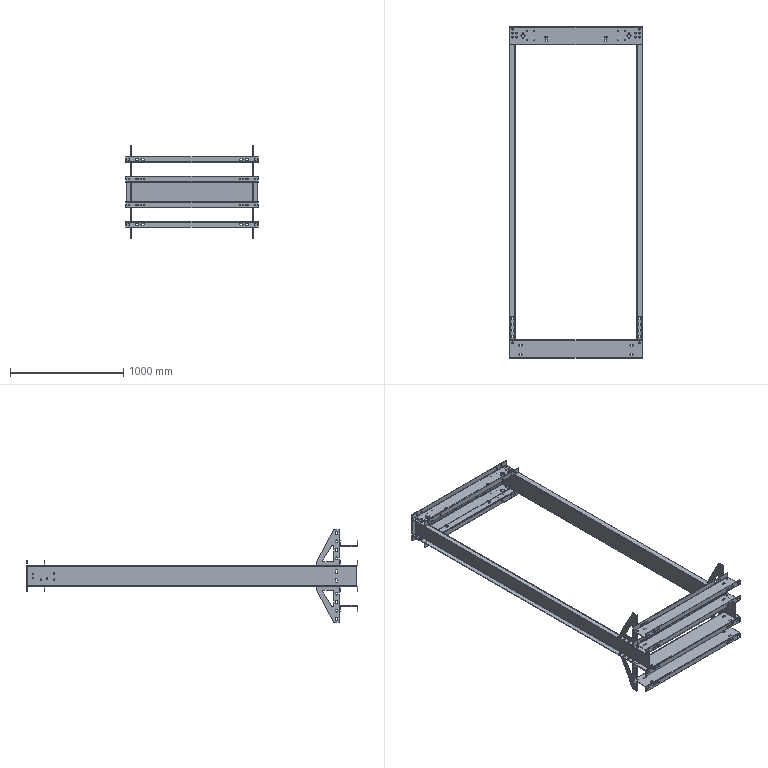Part | SolidWorks | features ReferencePattern 8, MirrorCompFeat 7 | 14 solids | 1176 faces | box 1170 x 2928 x 820 mm | volume 20192418 mm3 | cylinder 668 | plane 508 | commonest cylinder face diameters 13 x272 14 x140 12 x66 6 x48 8.5 x48 5 x24